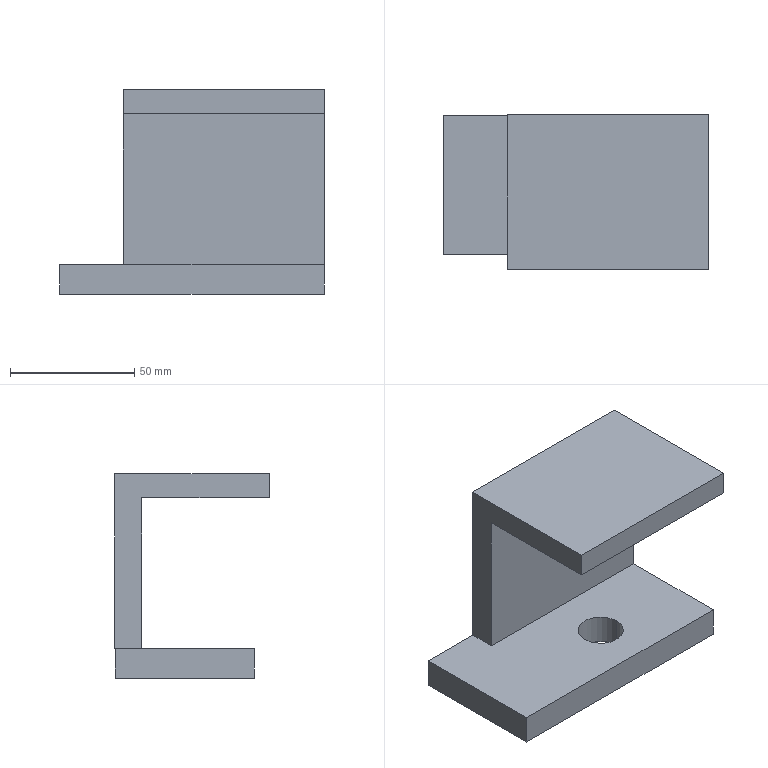Part | STEP file | Part 20 PN_0001_ASM 2 | 1 solid | 15 faces | box 106.46 x 62.346 x 82.377 mm | volume 171045 mm3 | plane 13 | cylinder 2 | commonest cylinder face diameters 18.213 x2
STEP:
#1=CARTESIAN_POINT('',(-222.34,-19.,0.));
#2=VERTEX_POINT('',#1);
#3=CARTESIAN_POINT('',(-204.127,-19.,0.));
#4=VERTEX_POINT('',#3);
#5=CARTESIAN_POINT('',(-213.233,-19.,0.));
#6=DIRECTION('',(0.,0.,1.));
#7=DIRECTION('',(1.,0.,0.));
#8=AXIS2_PLACEMENT_3D('',#5,#6,#7);
#9=CIRCLE('',#8,9.106);
#10=EDGE_CURVE('',#2,#4,#9,.T.);
#11=ORIENTED_EDGE('',*,*,#10,.F.);
#12=CARTESIAN_POINT('',(-222.34,-19.,12.));
#13=VERTEX_POINT('',#12);
#14=CARTESIAN_POINT('',(-222.34,-19.,0.));
#15=DIRECTION('',(0.,0.,1.));
#16=VECTOR('',#15,1000.);
#17=LINE('',#14,#16);
#18=EDGE_CURVE('',#2,#13,#17,.T.);
#19=ORIENTED_EDGE('',*,*,#18,.T.);
#20=CARTESIAN_POINT('',(-204.127,-19.,12.));
#21=VERTEX_POINT('',#20);
#22=CARTESIAN_POINT('',(-213.233,-19.,12.));
#23=DIRECTION('',(0.,0.,1.));
#24=DIRECTION('',(1.,0.,0.));
#25=AXIS2_PLACEMENT_3D('',#22,#23,#24);
#26=CIRCLE('',#25,9.106);
#27=EDGE_CURVE('',#13,#21,#26,.T.);
#28=ORIENTED_EDGE('',*,*,#27,.T.);
#29=CARTESIAN_POINT('',(-204.127,-19.,0.));
#30=DIRECTION('',(0.,0.,1.));
#31=VECTOR('',#30,1000.);
#32=LINE('',#29,#31);
#33=EDGE_CURVE('',#4,#21,#32,.T.);
#34=ORIENTED_EDGE('',*,*,#33,.F.);
#35=EDGE_LOOP('',(#11,#19,#28,#34));
#36=FACE_OUTER_BOUND('',#35,.T.);
#37=CARTESIAN_POINT('',(-213.233,-19.,0.));
#38=DIRECTION('',(0.,0.,1.));
#39=DIRECTION('',(1.,0.,0.));
#40=AXIS2_PLACEMENT_3D('',#37,#38,#39);
#41=CYLINDRICAL_SURFACE('',#40,9.106);
#42=ADVANCED_FACE('',(#36),#41,.F.);
#43=CARTESIAN_POINT('',(-213.233,-19.,12.));
#44=DIRECTION('',(0.,0.,1.));
#45=DIRECTION('',(1.,0.,0.));
#46=AXIS2_PLACEMENT_3D('',#43,#44,#45);
#47=CIRCLE('',#46,9.106);
#48=EDGE_CURVE('',#21,#13,#47,.T.);
#49=ORIENTED_EDGE('',*,*,#48,.F.);
#50=ORIENTED_EDGE('',*,*,#27,.F.);
#51=EDGE_LOOP('',(#49,#50));
#52=FACE_BOUND('',#51,.T.);
#53=CARTESIAN_POINT('',(-252.087,4.442,12.));
#54=VERTEX_POINT('',#53);
#55=CARTESIAN_POINT('',(-171.087,4.442,12.));
#56=VERTEX_POINT('',#55);
#57=CARTESIAN_POINT('',(-252.087,4.442,12.));
#58=DIRECTION('',(1.,0.,0.));
#59=VECTOR('',#58,1000.);
#60=LINE('',#57,#59);
#61=EDGE_CURVE('',#54,#56,#60,.T.);
#62=ORIENTED_EDGE('',*,*,#61,.F.);
#63=CARTESIAN_POINT('',(-252.087,15.,12.));
#64=VERTEX_POINT('',#63);
#65=CARTESIAN_POINT('',(-252.087,15.346,12.));
#66=DIRECTION('',(0.,1.,0.));
#67=VECTOR('',#66,1000.);
#68=LINE('',#65,#67);
#69=EDGE_CURVE('',#54,#64,#68,.T.);
#70=ORIENTED_EDGE('',*,*,#69,.T.);
#71=CARTESIAN_POINT('',(-277.547,15.,12.));
#72=VERTEX_POINT('',#71);
#73=CARTESIAN_POINT('',(-171.087,15.,12.));
#74=DIRECTION('',(-1.,0.,0.));
#75=VECTOR('',#74,1000.);
#76=LINE('',#73,#75);
#77=EDGE_CURVE('',#64,#72,#76,.T.);
#78=ORIENTED_EDGE('',*,*,#77,.T.);
#79=CARTESIAN_POINT('',(-277.547,-41.,12.));
#80=VERTEX_POINT('',#79);
#81=CARTESIAN_POINT('',(-277.547,15.,12.));
#82=DIRECTION('',(0.,-1.,0.));
#83=VECTOR('',#82,1000.);
#84=LINE('',#81,#83);
#85=EDGE_CURVE('',#72,#80,#84,.T.);
#86=ORIENTED_EDGE('',*,*,#85,.T.);
#87=CARTESIAN_POINT('',(-171.087,-41.,12.));
#88=VERTEX_POINT('',#87);
#89=CARTESIAN_POINT('',(-171.087,-41.,12.));
#90=DIRECTION('',(1.,0.,0.));
#91=VECTOR('',#90,1000.);
#92=LINE('',#89,#91);
#93=EDGE_CURVE('',#80,#88,#92,.T.);
#94=ORIENTED_EDGE('',*,*,#93,.T.);
#95=CARTESIAN_POINT('',(-171.087,15.,12.));
#96=DIRECTION('',(0.,1.,0.));
#97=VECTOR('',#96,1000.);
#98=LINE('',#95,#97);
#99=EDGE_CURVE('',#88,#56,#98,.T.);
#100=ORIENTED_EDGE('',*,*,#99,.T.);
#101=EDGE_LOOP('',(#62,#70,#78,#86,#94,#100));
#102=FACE_OUTER_BOUND('',#101,.T.);
#103=CARTESIAN_POINT('',(-171.087,-41.,12.));
#104=DIRECTION('',(0.,0.,-1.));
#105=DIRECTION('',(-1.,0.,0.));
#106=AXIS2_PLACEMENT_3D('',#103,#104,#105);
#107=PLANE('',#106);
#108=ADVANCED_FACE('',(#52,#102),#107,.F.);
#109=CARTESIAN_POINT('',(-171.087,-41.,0.));
#110=VERTEX_POINT('',#109);
#111=CARTESIAN_POINT('',(-171.087,15.,0.));
#112=VERTEX_POINT('',#111);
#113=CARTESIAN_POINT('',(-171.087,15.,0.));
#114=DIRECTION('',(0.,1.,0.));
#115=VECTOR('',#114,1000.);
#116=LINE('',#113,#115);
#117=EDGE_CURVE('',#110,#112,#116,.T.);
#118=ORIENTED_EDGE('',*,*,#117,.T.);
#119=CARTESIAN_POINT('',(-171.087,15.,12.));
#120=VERTEX_POINT('',#119);
#121=CARTESIAN_POINT('',(-171.087,15.,12.));
#122=DIRECTION('',(0.,0.,-1.));
#123=VECTOR('',#122,1000.);
#124=LINE('',#121,#123);
#125=EDGE_CURVE('',#120,#112,#124,.T.);
#126=ORIENTED_EDGE('',*,*,#125,.F.);
#127=CARTESIAN_POINT('',(-171.087,15.346,12.));
#128=VERTEX_POINT('',#127);
#129=CARTESIAN_POINT('',(-171.087,15.346,12.));
#130=DIRECTION('',(0.,1.,0.));
#131=VECTOR('',#130,1000.);
#132=LINE('',#129,#131);
#133=EDGE_CURVE('',#120,#128,#132,.T.);
#134=ORIENTED_EDGE('',*,*,#133,.T.);
#135=CARTESIAN_POINT('',(-171.087,15.346,82.377));
#136=VERTEX_POINT('',#135);
#137=CARTESIAN_POINT('',(-171.087,15.346,82.377));
#138=DIRECTION('',(0.,0.,1.));
#139=VECTOR('',#138,1000.);
#140=LINE('',#137,#139);
#141=EDGE_CURVE('',#128,#136,#140,.T.);
#142=ORIENTED_EDGE('',*,*,#141,.T.);
#143=CARTESIAN_POINT('',(-171.087,-47.,82.377));
#144=VERTEX_POINT('',#143);
#145=CARTESIAN_POINT('',(-171.087,-47.,82.377));
#146=DIRECTION('',(0.,-1.,0.));
#147=VECTOR('',#146,1000.);
#148=LINE('',#145,#147);
#149=EDGE_CURVE('',#136,#144,#148,.T.);
#150=ORIENTED_EDGE('',*,*,#149,.T.);
#151=CARTESIAN_POINT('',(-171.087,-47.,72.664));
#152=VERTEX_POINT('',#151);
#153=CARTESIAN_POINT('',(-171.087,-47.,82.377));
#154=DIRECTION('',(0.,0.,-1.));
#155=VECTOR('',#154,1000.);
#156=LINE('',#153,#155);
#157=EDGE_CURVE('',#144,#152,#156,.T.);
#158=ORIENTED_EDGE('',*,*,#157,.T.);
#159=CARTESIAN_POINT('',(-171.087,4.442,72.664));
#160=VERTEX_POINT('',#159);
#161=CARTESIAN_POINT('',(-171.087,-47.,72.664));
#162=DIRECTION('',(0.,1.,0.));
#163=VECTOR('',#162,1000.);
#164=LINE('',#161,#163);
#165=EDGE_CURVE('',#152,#160,#164,.T.);
#166=ORIENTED_EDGE('',*,*,#165,.T.);
#167=CARTESIAN_POINT('',(-171.087,4.442,72.664));
#168=DIRECTION('',(0.,0.,-1.));
#169=VECTOR('',#168,1000.);
#170=LINE('',#167,#169);
#171=EDGE_CURVE('',#160,#56,#170,.T.);
#172=ORIENTED_EDGE('',*,*,#171,.T.);
#173=ORIENTED_EDGE('',*,*,#99,.F.);
#174=CARTESIAN_POINT('',(-171.087,-41.,12.));
#175=DIRECTION('',(0.,0.,-1.));
#176=VECTOR('',#175,1000.);
#177=LINE('',#174,#176);
#178=EDGE_CURVE('',#88,#110,#177,.T.);
#179=ORIENTED_EDGE('',*,*,#178,.T.);
#180=EDGE_LOOP('',(#118,#126,#134,#142,#150,#158,#166,#172,#173,#179));
#181=FACE_OUTER_BOUND('',#180,.T.);
#182=CARTESIAN_POINT('',(-171.087,15.,12.));
#183=DIRECTION('',(-1.,0.,0.));
#184=DIRECTION('',(0.,0.,1.));
#185=AXIS2_PLACEMENT_3D('',#182,#183,#184);
#186=PLANE('',#185);
#187=ADVANCED_FACE('',(#181),#186,.F.);
#188=CARTESIAN_POINT('',(-277.547,15.,0.));
#189=VERTEX_POINT('',#188);
#190=CARTESIAN_POINT('',(-171.087,15.,0.));
#191=DIRECTION('',(-1.,0.,0.));
#192=VECTOR('',#191,1000.);
#193=LINE('',#190,#192);
#194=EDGE_CURVE('',#112,#189,#193,.T.);
#195=ORIENTED_EDGE('',*,*,#194,.T.);
#196=CARTESIAN_POINT('',(-277.547,15.,12.));
#197=DIRECTION('',(0.,0.,-1.));
#198=VECTOR('',#197,1000.);
#199=LINE('',#196,#198);
#200=EDGE_CURVE('',#72,#189,#199,.T.);
#201=ORIENTED_EDGE('',*,*,#200,.F.);
#202=ORIENTED_EDGE('',*,*,#77,.F.);
#203=CARTESIAN_POINT('',(-171.087,15.,12.));
#204=DIRECTION('',(-1.,0.,0.));
#205=VECTOR('',#204,1000.);
#206=LINE('',#203,#205);
#207=EDGE_CURVE('',#120,#64,#206,.T.);
#208=ORIENTED_EDGE('',*,*,#207,.F.);
#209=ORIENTED_EDGE('',*,*,#125,.T.);
#210=EDGE_LOOP('',(#195,#201,#202,#208,#209));
#211=FACE_OUTER_BOUND('',#210,.T.);
#212=CARTESIAN_POINT('',(-171.087,15.,12.));
#213=DIRECTION('',(0.,-1.,0.));
#214=DIRECTION('',(0.,0.,-1.));
#215=AXIS2_PLACEMENT_3D('',#212,#213,#214);
#216=PLANE('',#215);
#217=ADVANCED_FACE('',(#211),#216,.F.);
#218=CARTESIAN_POINT('',(-277.547,-41.,0.));
#219=VERTEX_POINT('',#218);
#220=CARTESIAN_POINT('',(-277.547,15.,0.));
#221=DIRECTION('',(0.,-1.,0.));
#222=VECTOR('',#221,1000.);
#223=LINE('',#220,#222);
#224=EDGE_CURVE('',#189,#219,#223,.T.);
#225=ORIENTED_EDGE('',*,*,#224,.T.);
#226=CARTESIAN_POINT('',(-277.547,-41.,12.));
#227=DIRECTION('',(0.,0.,-1.));
#228=VECTOR('',#227,1000.);
#229=LINE('',#226,#228);
#230=EDGE_CURVE('',#80,#219,#229,.T.);
#231=ORIENTED_EDGE('',*,*,#230,.F.);
#232=ORIENTED_EDGE('',*,*,#85,.F.);
#233=ORIENTED_EDGE('',*,*,#200,.T.);
#234=EDGE_LOOP('',(#225,#231,#232,#233));
#235=FACE_OUTER_BOUND('',#234,.T.);
#236=CARTESIAN_POINT('',(-277.547,15.,12.));
#237=DIRECTION('',(1.,0.,0.));
#238=DIRECTION('',(0.,0.,-1.));
#239=AXIS2_PLACEMENT_3D('',#236,#237,#238);
#240=PLANE('',#239);
#241=ADVANCED_FACE('',(#235),#240,.F.);
#242=CARTESIAN_POINT('',(-171.087,-41.,0.));
#243=DIRECTION('',(1.,0.,0.));
#244=VECTOR('',#243,1000.);
#245=LINE('',#242,#244);
#246=EDGE_CURVE('',#219,#110,#245,.T.);
#247=ORIENTED_EDGE('',*,*,#246,.T.);
#248=ORIENTED_EDGE('',*,*,#178,.F.);
#249=ORIENTED_EDGE('',*,*,#93,.F.);
#250=ORIENTED_EDGE('',*,*,#230,.T.);
#251=EDGE_LOOP('',(#247,#248,#249,#250));
#252=FACE_OUTER_BOUND('',#251,.T.);
#253=CARTESIAN_POINT('',(-171.087,-41.,12.));
#254=DIRECTION('',(0.,1.,0.));
#255=DIRECTION('',(0.,0.,1.));
#256=AXIS2_PLACEMENT_3D('',#253,#254,#255);
#257=PLANE('',#256);
#258=ADVANCED_FACE('',(#252),#257,.F.);
#259=CARTESIAN_POINT('',(-213.233,-19.,0.));
#260=DIRECTION('',(0.,0.,1.));
#261=DIRECTION('',(1.,0.,0.));
#262=AXIS2_PLACEMENT_3D('',#259,#260,#261);
#263=CIRCLE('',#262,9.106);
#264=EDGE_CURVE('',#4,#2,#263,.T.);
#265=ORIENTED_EDGE('',*,*,#264,.T.);
#266=ORIENTED_EDGE('',*,*,#10,.T.);
#267=EDGE_LOOP('',(#265,#266));
#268=FACE_BOUND('',#267,.T.);
#269=ORIENTED_EDGE('',*,*,#117,.F.);
#270=ORIENTED_EDGE('',*,*,#246,.F.);
#271=ORIENTED_EDGE('',*,*,#224,.F.);
#272=ORIENTED_EDGE('',*,*,#194,.F.);
#273=EDGE_LOOP('',(#269,#270,#271,#272));
#274=FACE_OUTER_BOUND('',#273,.T.);
#275=CARTESIAN_POINT('',(-171.087,-41.,0.));
#276=DIRECTION('',(0.,0.,-1.));
#277=DIRECTION('',(-1.,0.,0.));
#278=AXIS2_PLACEMENT_3D('',#275,#276,#277);
#279=PLANE('',#278);
#280=ADVANCED_FACE('',(#268,#274),#279,.T.);
#281=ORIENTED_EDGE('',*,*,#18,.F.);
#282=ORIENTED_EDGE('',*,*,#264,.F.);
#283=ORIENTED_EDGE('',*,*,#33,.T.);
#284=ORIENTED_EDGE('',*,*,#48,.T.);
#285=EDGE_LOOP('',(#281,#282,#283,#284));
#286=FACE_OUTER_BOUND('',#285,.T.);
#287=CARTESIAN_POINT('',(-213.233,-19.,0.));
#288=DIRECTION('',(0.,0.,1.));
#289=DIRECTION('',(1.,0.,0.));
#290=AXIS2_PLACEMENT_3D('',#287,#288,#289);
#291=CYLINDRICAL_SURFACE('',#290,9.106);
#292=ADVANCED_FACE('',(#286),#291,.F.);
#293=ORIENTED_EDGE('',*,*,#149,.F.);
#294=CARTESIAN_POINT('',(-252.087,15.346,82.377));
#295=VERTEX_POINT('',#294);
#296=CARTESIAN_POINT('',(-252.087,15.346,82.377));
#297=DIRECTION('',(1.,0.,0.));
#298=VECTOR('',#297,1000.);
#299=LINE('',#296,#298);
#300=EDGE_CURVE('',#295,#136,#299,.T.);
#301=ORIENTED_EDGE('',*,*,#300,.F.);
#302=CARTESIAN_POINT('',(-252.087,-47.,82.377));
#303=VERTEX_POINT('',#302);
#304=CARTESIAN_POINT('',(-252.087,-47.,82.377));
#305=DIRECTION('',(0.,-1.,0.));
#306=VECTOR('',#305,1000.);
#307=LINE('',#304,#306);
#308=EDGE_CURVE('',#295,#303,#307,.T.);
#309=ORIENTED_EDGE('',*,*,#308,.T.);
#310=CARTESIAN_POINT('',(-252.087,-47.,82.377));
#311=DIRECTION('',(1.,0.,0.));
#312=VECTOR('',#311,1000.);
#313=LINE('',#310,#312);
#314=EDGE_CURVE('',#303,#144,#313,.T.);
#315=ORIENTED_EDGE('',*,*,#314,.T.);
#316=EDGE_LOOP('',(#293,#301,#309,#315));
#317=FACE_OUTER_BOUND('',#316,.T.);
#318=CARTESIAN_POINT('',(-252.087,-47.,82.377));
#319=DIRECTION('',(0.,0.,1.));
#320=DIRECTION('',(1.,0.,0.));
#321=AXIS2_PLACEMENT_3D('',#318,#319,#320);
#322=PLANE('',#321);
#323=ADVANCED_FACE('',(#317),#322,.T.);
#324=ORIENTED_EDGE('',*,*,#141,.F.);
#325=CARTESIAN_POINT('',(-252.087,15.346,12.));
#326=VERTEX_POINT('',#325);
#327=CARTESIAN_POINT('',(-252.087,15.346,12.));
#328=DIRECTION('',(1.,0.,0.));
#329=VECTOR('',#328,1000.);
#330=LINE('',#327,#329);
#331=EDGE_CURVE('',#326,#128,#330,.T.);
#332=ORIENTED_EDGE('',*,*,#331,.F.);
#333=CARTESIAN_POINT('',(-252.087,15.346,72.664));
#334=DIRECTION('',(0.,0.,1.));
#335=VECTOR('',#334,1000.);
#336=LINE('',#333,#335);
#337=EDGE_CURVE('',#326,#295,#336,.T.);
#338=ORIENTED_EDGE('',*,*,#337,.T.);
#339=ORIENTED_EDGE('',*,*,#300,.T.);
#340=EDGE_LOOP('',(#324,#332,#338,#339));
#341=FACE_OUTER_BOUND('',#340,.T.);
#342=CARTESIAN_POINT('',(-252.087,15.346,82.377));
#343=DIRECTION('',(0.,1.,0.));
#344=DIRECTION('',(0.,0.,1.));
#345=AXIS2_PLACEMENT_3D('',#342,#343,#344);
#346=PLANE('',#345);
#347=ADVANCED_FACE('',(#341),#346,.T.);
#348=ORIENTED_EDGE('',*,*,#133,.F.);
#349=ORIENTED_EDGE('',*,*,#207,.T.);
#350=CARTESIAN_POINT('',(-252.087,15.346,12.));
#351=DIRECTION('',(0.,1.,0.));
#352=VECTOR('',#351,1000.);
#353=LINE('',#350,#352);
#354=EDGE_CURVE('',#64,#326,#353,.T.);
#355=ORIENTED_EDGE('',*,*,#354,.T.);
#356=ORIENTED_EDGE('',*,*,#331,.T.);
#357=EDGE_LOOP('',(#348,#349,#355,#356));
#358=FACE_OUTER_BOUND('',#357,.T.);
#359=CARTESIAN_POINT('',(-252.087,15.346,12.));
#360=DIRECTION('',(0.,0.,-1.));
#361=DIRECTION('',(-1.,0.,0.));
#362=AXIS2_PLACEMENT_3D('',#359,#360,#361);
#363=PLANE('',#362);
#364=ADVANCED_FACE('',(#358),#363,.T.);
#365=ORIENTED_EDGE('',*,*,#171,.F.);
#366=CARTESIAN_POINT('',(-252.087,4.442,72.664));
#367=VERTEX_POINT('',#366);
#368=CARTESIAN_POINT('',(-252.087,4.442,72.664));
#369=DIRECTION('',(1.,0.,0.));
#370=VECTOR('',#369,1000.);
#371=LINE('',#368,#370);
#372=EDGE_CURVE('',#367,#160,#371,.T.);
#373=ORIENTED_EDGE('',*,*,#372,.F.);
#374=CARTESIAN_POINT('',(-252.087,4.442,72.664));
#375=DIRECTION('',(0.,0.,-1.));
#376=VECTOR('',#375,1000.);
#377=LINE('',#374,#376);
#378=EDGE_CURVE('',#367,#54,#377,.T.);
#379=ORIENTED_EDGE('',*,*,#378,.T.);
#380=ORIENTED_EDGE('',*,*,#61,.T.);
#381=EDGE_LOOP('',(#365,#373,#379,#380));
#382=FACE_OUTER_BOUND('',#381,.T.);
#383=CARTESIAN_POINT('',(-252.087,4.442,72.664));
#384=DIRECTION('',(0.,-1.,0.));
#385=DIRECTION('',(0.,0.,-1.));
#386=AXIS2_PLACEMENT_3D('',#383,#384,#385);
#387=PLANE('',#386);
#388=ADVANCED_FACE('',(#382),#387,.T.);
#389=ORIENTED_EDGE('',*,*,#165,.F.);
#390=CARTESIAN_POINT('',(-252.087,-47.,72.664));
#391=VERTEX_POINT('',#390);
#392=CARTESIAN_POINT('',(-252.087,-47.,72.664));
#393=DIRECTION('',(1.,0.,0.));
#394=VECTOR('',#393,1000.);
#395=LINE('',#392,#394);
#396=EDGE_CURVE('',#391,#152,#395,.T.);
#397=ORIENTED_EDGE('',*,*,#396,.F.);
#398=CARTESIAN_POINT('',(-252.087,-47.,72.664));
#399=DIRECTION('',(0.,1.,0.));
#400=VECTOR('',#399,1000.);
#401=LINE('',#398,#400);
#402=EDGE_CURVE('',#391,#367,#401,.T.);
#403=ORIENTED_EDGE('',*,*,#402,.T.);
#404=ORIENTED_EDGE('',*,*,#372,.T.);
#405=EDGE_LOOP('',(#389,#397,#403,#404));
#406=FACE_OUTER_BOUND('',#405,.T.);
#407=CARTESIAN_POINT('',(-252.087,-47.,72.664));
#408=DIRECTION('',(0.,0.,-1.));
#409=DIRECTION('',(-1.,0.,0.));
#410=AXIS2_PLACEMENT_3D('',#407,#408,#409);
#411=PLANE('',#410);
#412=ADVANCED_FACE('',(#406),#411,.T.);
#413=ORIENTED_EDGE('',*,*,#157,.F.);
#414=ORIENTED_EDGE('',*,*,#314,.F.);
#415=CARTESIAN_POINT('',(-252.087,-47.,82.377));
#416=DIRECTION('',(0.,0.,-1.));
#417=VECTOR('',#416,1000.);
#418=LINE('',#415,#417);
#419=EDGE_CURVE('',#303,#391,#418,.T.);
#420=ORIENTED_EDGE('',*,*,#419,.T.);
#421=ORIENTED_EDGE('',*,*,#396,.T.);
#422=EDGE_LOOP('',(#413,#414,#420,#421));
#423=FACE_OUTER_BOUND('',#422,.T.);
#424=CARTESIAN_POINT('',(-252.087,-47.,82.377));
#425=DIRECTION('',(0.,-1.,0.));
#426=DIRECTION('',(0.,0.,-1.));
#427=AXIS2_PLACEMENT_3D('',#424,#425,#426);
#428=PLANE('',#427);
#429=ADVANCED_FACE('',(#423),#428,.T.);
#430=ORIENTED_EDGE('',*,*,#308,.F.);
#431=ORIENTED_EDGE('',*,*,#337,.F.);
#432=ORIENTED_EDGE('',*,*,#354,.F.);
#433=ORIENTED_EDGE('',*,*,#69,.F.);
#434=ORIENTED_EDGE('',*,*,#378,.F.);
#435=ORIENTED_EDGE('',*,*,#402,.F.);
#436=ORIENTED_EDGE('',*,*,#419,.F.);
#437=EDGE_LOOP('',(#430,#431,#432,#433,#434,#435,#436));
#438=FACE_OUTER_BOUND('',#437,.T.);
#439=CARTESIAN_POINT('',(-252.087,15.346,82.377));
#440=DIRECTION('',(-1.,0.,0.));
#441=DIRECTION('',(0.,0.,1.));
#442=AXIS2_PLACEMENT_3D('',#439,#440,#441);
#443=PLANE('',#442);
#444=ADVANCED_FACE('',(#438),#443,.T.);
#445=CLOSED_SHELL('',(#42,#108,#187,#217,#241,#258,#280,#292,#323,#347,#364,#388,#412,#429,#444));
#446=MANIFOLD_SOLID_BREP('',#445);
#447=CARTESIAN_POINT('',(0.,0.,0.));
#448=DIRECTION('',(0.,0.,1.));
#449=DIRECTION('',(1.,0.,0.));
#450=AXIS2_PLACEMENT_3D('',#447,#448,#449);
#451=(LENGTH_UNIT()NAMED_UNIT(*)SI_UNIT(.MILLI.,.METRE.));
#452=UNCERTAINTY_MEASURE_WITH_UNIT(LENGTH_MEASURE(0.00001),#451,'','');
#453=(NAMED_UNIT(*)PLANE_ANGLE_UNIT()SI_UNIT($,.RADIAN.));
#454=(NAMED_UNIT(*)SI_UNIT($,.STERADIAN.)SOLID_ANGLE_UNIT());
#455=(GEOMETRIC_REPRESENTATION_CONTEXT(3)GLOBAL_UNCERTAINTY_ASSIGNED_CONTEXT((#452))GLOBAL_UNIT_ASSIGNED_CONTEXT((#451,#453,#454))REPRESENTATION_CONTEXT('',''));
#456=ADVANCED_BREP_SHAPE_REPRESENTATION('',(#446,#450),#455);